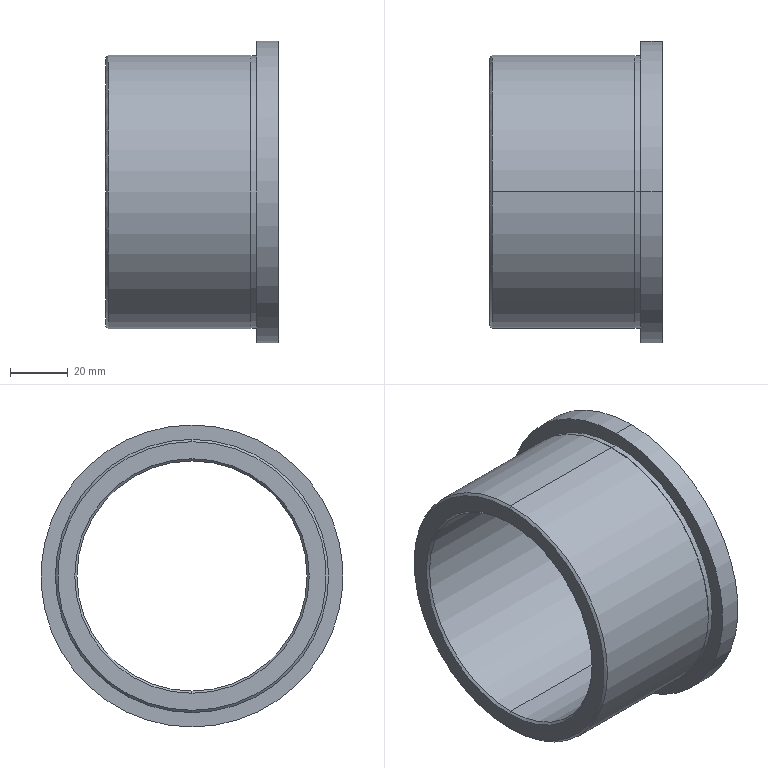Part | SolidWorks | features Revolution 1 | 1 solid | 18 faces | box 60 x 105 x 105 mm | volume 135111 mm3 | cylinder 8 | cone 6 | plane 4 | commonest cylinder face diameters 80 x2 94.6 x2 95 x2 105 x2
STEP:
#1=CARTESIAN_POINT('',(-30.,0.,46.7));
#2=VERTEX_POINT('',#1);
#3=CARTESIAN_POINT('',(-30.,0.,-46.7));
#4=VERTEX_POINT('',#3);
#5=CARTESIAN_POINT('',(-30.,0.,0.));
#6=DIRECTION('',(-1.,0.,0.));
#7=DIRECTION('',(0.,0.,1.));
#8=AXIS2_PLACEMENT_3D('',#5,#6,#7);
#9=CIRCLE('',#8,46.7);
#10=EDGE_CURVE('',#2,#4,#9,.T.);
#11=ORIENTED_EDGE('',*,*,#10,.F.);
#12=CARTESIAN_POINT('',(-29.2,0.,47.5));
#13=VERTEX_POINT('',#12);
#14=CARTESIAN_POINT('',(-29.2,0.,47.5));
#15=DIRECTION('',(0.7071,0.,0.7071));
#16=VECTOR('',#15,1000.);
#17=LINE('',#14,#16);
#18=EDGE_CURVE('',#2,#13,#17,.T.);
#19=ORIENTED_EDGE('',*,*,#18,.T.);
#20=CARTESIAN_POINT('',(-29.2,0.,-47.5));
#21=VERTEX_POINT('',#20);
#22=CARTESIAN_POINT('',(-29.2,0.,0.));
#23=DIRECTION('',(-1.,0.,0.));
#24=DIRECTION('',(0.,0.,1.));
#25=AXIS2_PLACEMENT_3D('',#22,#23,#24);
#26=CIRCLE('',#25,47.5);
#27=EDGE_CURVE('',#13,#21,#26,.T.);
#28=ORIENTED_EDGE('',*,*,#27,.T.);
#29=CARTESIAN_POINT('',(-29.2,0.,-47.5));
#30=DIRECTION('',(0.7071,0.,-0.7071));
#31=VECTOR('',#30,1000.);
#32=LINE('',#29,#31);
#33=EDGE_CURVE('',#4,#21,#32,.T.);
#34=ORIENTED_EDGE('',*,*,#33,.F.);
#35=EDGE_LOOP('',(#11,#19,#28,#34));
#36=FACE_OUTER_BOUND('',#35,.T.);
#37=CARTESIAN_POINT('',(-29.2,0.,0.));
#38=DIRECTION('',(1.,0.,0.));
#39=DIRECTION('',(0.,0.,-1.));
#40=AXIS2_PLACEMENT_3D('',#37,#38,#39);
#41=CONICAL_SURFACE('',#40,47.5,0.7854);
#42=ADVANCED_FACE('',(#36),#41,.T.);
#43=CARTESIAN_POINT('',(20.5,0.,47.5));
#44=VERTEX_POINT('',#43);
#45=CARTESIAN_POINT('',(20.5,0.,-47.5));
#46=VERTEX_POINT('',#45);
#47=CARTESIAN_POINT('',(20.5,0.,0.));
#48=DIRECTION('',(-1.,0.,0.));
#49=DIRECTION('',(0.,0.,1.));
#50=AXIS2_PLACEMENT_3D('',#47,#48,#49);
#51=CIRCLE('',#50,47.5);
#52=EDGE_CURVE('',#44,#46,#51,.T.);
#53=ORIENTED_EDGE('',*,*,#52,.T.);
#54=CARTESIAN_POINT('',(-30.,0.,-47.5));
#55=DIRECTION('',(-1.,0.,0.));
#56=VECTOR('',#55,1000.);
#57=LINE('',#54,#56);
#58=EDGE_CURVE('',#46,#21,#57,.T.);
#59=ORIENTED_EDGE('',*,*,#58,.T.);
#60=ORIENTED_EDGE('',*,*,#27,.F.);
#61=CARTESIAN_POINT('',(-30.,0.,47.5));
#62=DIRECTION('',(-1.,0.,0.));
#63=VECTOR('',#62,1000.);
#64=LINE('',#61,#63);
#65=EDGE_CURVE('',#44,#13,#64,.T.);
#66=ORIENTED_EDGE('',*,*,#65,.F.);
#67=EDGE_LOOP('',(#53,#59,#60,#66));
#68=FACE_OUTER_BOUND('',#67,.T.);
#69=CARTESIAN_POINT('',(-30.,0.,0.));
#70=DIRECTION('',(-1.,0.,0.));
#71=DIRECTION('',(0.,0.,1.));
#72=AXIS2_PLACEMENT_3D('',#69,#70,#71);
#73=CYLINDRICAL_SURFACE('',#72,47.5);
#74=ADVANCED_FACE('',(#68),#73,.T.);
#75=CARTESIAN_POINT('',(22.5,0.,47.3));
#76=VERTEX_POINT('',#75);
#77=CARTESIAN_POINT('',(22.5,0.,-47.3));
#78=VERTEX_POINT('',#77);
#79=CARTESIAN_POINT('',(22.5,0.,0.));
#80=DIRECTION('',(-1.,0.,0.));
#81=DIRECTION('',(0.,0.,1.));
#82=AXIS2_PLACEMENT_3D('',#79,#80,#81);
#83=CIRCLE('',#82,47.3);
#84=EDGE_CURVE('',#76,#78,#83,.T.);
#85=ORIENTED_EDGE('',*,*,#84,.T.);
#86=CARTESIAN_POINT('',(20.5,0.,-47.3));
#87=VERTEX_POINT('',#86);
#88=CARTESIAN_POINT('',(-30.,0.,-47.3));
#89=DIRECTION('',(-1.,0.,0.));
#90=VECTOR('',#89,1000.);
#91=LINE('',#88,#90);
#92=EDGE_CURVE('',#78,#87,#91,.T.);
#93=ORIENTED_EDGE('',*,*,#92,.T.);
#94=CARTESIAN_POINT('',(20.5,0.,47.3));
#95=VERTEX_POINT('',#94);
#96=CARTESIAN_POINT('',(20.5,0.,0.));
#97=DIRECTION('',(-1.,0.,0.));
#98=DIRECTION('',(0.,0.,1.));
#99=AXIS2_PLACEMENT_3D('',#96,#97,#98);
#100=CIRCLE('',#99,47.3);
#101=EDGE_CURVE('',#95,#87,#100,.T.);
#102=ORIENTED_EDGE('',*,*,#101,.F.);
#103=CARTESIAN_POINT('',(-30.,0.,47.3));
#104=DIRECTION('',(-1.,0.,0.));
#105=VECTOR('',#104,1000.);
#106=LINE('',#103,#105);
#107=EDGE_CURVE('',#76,#95,#106,.T.);
#108=ORIENTED_EDGE('',*,*,#107,.F.);
#109=EDGE_LOOP('',(#85,#93,#102,#108));
#110=FACE_OUTER_BOUND('',#109,.T.);
#111=CARTESIAN_POINT('',(-30.,0.,0.));
#112=DIRECTION('',(-1.,0.,0.));
#113=DIRECTION('',(0.,0.,1.));
#114=AXIS2_PLACEMENT_3D('',#111,#112,#113);
#115=CYLINDRICAL_SURFACE('',#114,47.3);
#116=ADVANCED_FACE('',(#110),#115,.T.);
#117=CARTESIAN_POINT('',(30.,0.,52.5));
#118=VERTEX_POINT('',#117);
#119=CARTESIAN_POINT('',(30.,0.,-52.5));
#120=VERTEX_POINT('',#119);
#121=CARTESIAN_POINT('',(30.,0.,0.));
#122=DIRECTION('',(-1.,0.,0.));
#123=DIRECTION('',(0.,0.,1.));
#124=AXIS2_PLACEMENT_3D('',#121,#122,#123);
#125=CIRCLE('',#124,52.5);
#126=EDGE_CURVE('',#118,#120,#125,.T.);
#127=ORIENTED_EDGE('',*,*,#126,.T.);
#128=CARTESIAN_POINT('',(22.5,0.,-52.5));
#129=VERTEX_POINT('',#128);
#130=CARTESIAN_POINT('',(-30.,0.,-52.5));
#131=DIRECTION('',(-1.,0.,0.));
#132=VECTOR('',#131,1000.);
#133=LINE('',#130,#132);
#134=EDGE_CURVE('',#120,#129,#133,.T.);
#135=ORIENTED_EDGE('',*,*,#134,.T.);
#136=CARTESIAN_POINT('',(22.5,0.,52.5));
#137=VERTEX_POINT('',#136);
#138=CARTESIAN_POINT('',(22.5,0.,0.));
#139=DIRECTION('',(-1.,0.,0.));
#140=DIRECTION('',(0.,0.,1.));
#141=AXIS2_PLACEMENT_3D('',#138,#139,#140);
#142=CIRCLE('',#141,52.5);
#143=EDGE_CURVE('',#137,#129,#142,.T.);
#144=ORIENTED_EDGE('',*,*,#143,.F.);
#145=CARTESIAN_POINT('',(-30.,0.,52.5));
#146=DIRECTION('',(-1.,0.,0.));
#147=VECTOR('',#146,1000.);
#148=LINE('',#145,#147);
#149=EDGE_CURVE('',#118,#137,#148,.T.);
#150=ORIENTED_EDGE('',*,*,#149,.F.);
#151=EDGE_LOOP('',(#127,#135,#144,#150));
#152=FACE_OUTER_BOUND('',#151,.T.);
#153=CARTESIAN_POINT('',(-30.,0.,0.));
#154=DIRECTION('',(-1.,0.,0.));
#155=DIRECTION('',(0.,0.,1.));
#156=AXIS2_PLACEMENT_3D('',#153,#154,#155);
#157=CYLINDRICAL_SURFACE('',#156,52.5);
#158=ADVANCED_FACE('',(#152),#157,.T.);
#159=CARTESIAN_POINT('',(29.2,0.,-40.));
#160=VERTEX_POINT('',#159);
#161=CARTESIAN_POINT('',(29.2,0.,40.));
#162=VERTEX_POINT('',#161);
#163=CARTESIAN_POINT('',(29.2,0.,0.));
#164=DIRECTION('',(-1.,0.,0.));
#165=DIRECTION('',(0.,0.,1.));
#166=AXIS2_PLACEMENT_3D('',#163,#164,#165);
#167=CIRCLE('',#166,40.);
#168=EDGE_CURVE('',#160,#162,#167,.T.);
#169=ORIENTED_EDGE('',*,*,#168,.T.);
#170=CARTESIAN_POINT('',(30.,0.,40.773));
#171=VERTEX_POINT('',#170);
#172=CARTESIAN_POINT('',(29.2,0.,40.));
#173=DIRECTION('',(0.7193,0.,0.6947));
#174=VECTOR('',#173,1000.);
#175=LINE('',#172,#174);
#176=EDGE_CURVE('',#162,#171,#175,.T.);
#177=ORIENTED_EDGE('',*,*,#176,.T.);
#178=CARTESIAN_POINT('',(30.,0.,-40.773));
#179=VERTEX_POINT('',#178);
#180=CARTESIAN_POINT('',(30.,0.,0.));
#181=DIRECTION('',(-1.,0.,0.));
#182=DIRECTION('',(0.,0.,1.));
#183=AXIS2_PLACEMENT_3D('',#180,#181,#182);
#184=CIRCLE('',#183,40.773);
#185=EDGE_CURVE('',#179,#171,#184,.T.);
#186=ORIENTED_EDGE('',*,*,#185,.F.);
#187=CARTESIAN_POINT('',(29.2,0.,-40.));
#188=DIRECTION('',(0.7193,0.,-0.6947));
#189=VECTOR('',#188,1000.);
#190=LINE('',#187,#189);
#191=EDGE_CURVE('',#160,#179,#190,.T.);
#192=ORIENTED_EDGE('',*,*,#191,.F.);
#193=EDGE_LOOP('',(#169,#177,#186,#192));
#194=FACE_OUTER_BOUND('',#193,.T.);
#195=CARTESIAN_POINT('',(29.2,0.,0.));
#196=DIRECTION('',(1.,0.,0.));
#197=DIRECTION('',(0.,0.,-1.));
#198=AXIS2_PLACEMENT_3D('',#195,#196,#197);
#199=CONICAL_SURFACE('',#198,40.,0.7679);
#200=ADVANCED_FACE('',(#194),#199,.F.);
#201=ORIENTED_EDGE('',*,*,#168,.F.);
#202=CARTESIAN_POINT('',(-29.2,0.,-40.));
#203=VERTEX_POINT('',#202);
#204=CARTESIAN_POINT('',(-30.,0.,-40.));
#205=DIRECTION('',(-1.,0.,0.));
#206=VECTOR('',#205,1000.);
#207=LINE('',#204,#206);
#208=EDGE_CURVE('',#160,#203,#207,.T.);
#209=ORIENTED_EDGE('',*,*,#208,.T.);
#210=CARTESIAN_POINT('',(-29.2,0.,40.));
#211=VERTEX_POINT('',#210);
#212=CARTESIAN_POINT('',(-29.2,0.,0.));
#213=DIRECTION('',(-1.,0.,0.));
#214=DIRECTION('',(0.,0.,1.));
#215=AXIS2_PLACEMENT_3D('',#212,#213,#214);
#216=CIRCLE('',#215,40.);
#217=EDGE_CURVE('',#203,#211,#216,.T.);
#218=ORIENTED_EDGE('',*,*,#217,.T.);
#219=CARTESIAN_POINT('',(-30.,0.,40.));
#220=DIRECTION('',(-1.,0.,0.));
#221=VECTOR('',#220,1000.);
#222=LINE('',#219,#221);
#223=EDGE_CURVE('',#162,#211,#222,.T.);
#224=ORIENTED_EDGE('',*,*,#223,.F.);
#225=EDGE_LOOP('',(#201,#209,#218,#224));
#226=FACE_OUTER_BOUND('',#225,.T.);
#227=CARTESIAN_POINT('',(-30.,0.,0.));
#228=DIRECTION('',(-1.,0.,0.));
#229=DIRECTION('',(0.,0.,1.));
#230=AXIS2_PLACEMENT_3D('',#227,#228,#229);
#231=CYLINDRICAL_SURFACE('',#230,40.);
#232=ADVANCED_FACE('',(#226),#231,.F.);
#233=ORIENTED_EDGE('',*,*,#217,.F.);
#234=CARTESIAN_POINT('',(-30.,0.,-40.773));
#235=VERTEX_POINT('',#234);
#236=CARTESIAN_POINT('',(-30.,0.,-40.773));
#237=DIRECTION('',(-0.7193,0.,-0.6947));
#238=VECTOR('',#237,1000.);
#239=LINE('',#236,#238);
#240=EDGE_CURVE('',#203,#235,#239,.T.);
#241=ORIENTED_EDGE('',*,*,#240,.T.);
#242=CARTESIAN_POINT('',(-30.,0.,40.773));
#243=VERTEX_POINT('',#242);
#244=CARTESIAN_POINT('',(-30.,0.,0.));
#245=DIRECTION('',(-1.,0.,0.));
#246=DIRECTION('',(0.,0.,1.));
#247=AXIS2_PLACEMENT_3D('',#244,#245,#246);
#248=CIRCLE('',#247,40.773);
#249=EDGE_CURVE('',#235,#243,#248,.T.);
#250=ORIENTED_EDGE('',*,*,#249,.T.);
#251=CARTESIAN_POINT('',(-30.,0.,40.773));
#252=DIRECTION('',(-0.7193,0.,0.6947));
#253=VECTOR('',#252,1000.);
#254=LINE('',#251,#253);
#255=EDGE_CURVE('',#211,#243,#254,.T.);
#256=ORIENTED_EDGE('',*,*,#255,.F.);
#257=EDGE_LOOP('',(#233,#241,#250,#256));
#258=FACE_OUTER_BOUND('',#257,.T.);
#259=CARTESIAN_POINT('',(-30.,0.,0.));
#260=DIRECTION('',(-1.,0.,0.));
#261=DIRECTION('',(0.,0.,1.));
#262=AXIS2_PLACEMENT_3D('',#259,#260,#261);
#263=CONICAL_SURFACE('',#262,40.773,0.7679);
#264=ADVANCED_FACE('',(#258),#263,.F.);
#265=CARTESIAN_POINT('',(-30.,0.,0.));
#266=DIRECTION('',(-1.,0.,0.));
#267=DIRECTION('',(0.,0.,1.));
#268=AXIS2_PLACEMENT_3D('',#265,#266,#267);
#269=CIRCLE('',#268,40.773);
#270=EDGE_CURVE('',#243,#235,#269,.T.);
#271=ORIENTED_EDGE('',*,*,#270,.F.);
#272=ORIENTED_EDGE('',*,*,#249,.F.);
#273=EDGE_LOOP('',(#271,#272));
#274=FACE_BOUND('',#273,.T.);
#275=CARTESIAN_POINT('',(-30.,0.,0.));
#276=DIRECTION('',(-1.,0.,0.));
#277=DIRECTION('',(0.,0.,1.));
#278=AXIS2_PLACEMENT_3D('',#275,#276,#277);
#279=CIRCLE('',#278,46.7);
#280=EDGE_CURVE('',#4,#2,#279,.T.);
#281=ORIENTED_EDGE('',*,*,#280,.T.);
#282=ORIENTED_EDGE('',*,*,#10,.T.);
#283=EDGE_LOOP('',(#281,#282));
#284=FACE_OUTER_BOUND('',#283,.T.);
#285=CARTESIAN_POINT('',(-30.,46.7,0.));
#286=DIRECTION('',(1.,0.,0.));
#287=DIRECTION('',(0.,0.,-1.));
#288=AXIS2_PLACEMENT_3D('',#285,#286,#287);
#289=PLANE('',#288);
#290=ADVANCED_FACE('',(#274,#284),#289,.F.);
#291=ORIENTED_EDGE('',*,*,#240,.F.);
#292=CARTESIAN_POINT('',(-29.2,0.,0.));
#293=DIRECTION('',(-1.,0.,0.));
#294=DIRECTION('',(0.,0.,1.));
#295=AXIS2_PLACEMENT_3D('',#292,#293,#294);
#296=CIRCLE('',#295,40.);
#297=EDGE_CURVE('',#211,#203,#296,.T.);
#298=ORIENTED_EDGE('',*,*,#297,.F.);
#299=ORIENTED_EDGE('',*,*,#255,.T.);
#300=ORIENTED_EDGE('',*,*,#270,.T.);
#301=EDGE_LOOP('',(#291,#298,#299,#300));
#302=FACE_OUTER_BOUND('',#301,.T.);
#303=CARTESIAN_POINT('',(-30.,0.,0.));
#304=DIRECTION('',(-1.,0.,0.));
#305=DIRECTION('',(0.,0.,1.));
#306=AXIS2_PLACEMENT_3D('',#303,#304,#305);
#307=CONICAL_SURFACE('',#306,40.773,0.7679);
#308=ADVANCED_FACE('',(#302),#307,.F.);
#309=ORIENTED_EDGE('',*,*,#208,.F.);
#310=CARTESIAN_POINT('',(29.2,0.,0.));
#311=DIRECTION('',(-1.,0.,0.));
#312=DIRECTION('',(0.,0.,1.));
#313=AXIS2_PLACEMENT_3D('',#310,#311,#312);
#314=CIRCLE('',#313,40.);
#315=EDGE_CURVE('',#162,#160,#314,.T.);
#316=ORIENTED_EDGE('',*,*,#315,.F.);
#317=ORIENTED_EDGE('',*,*,#223,.T.);
#318=ORIENTED_EDGE('',*,*,#297,.T.);
#319=EDGE_LOOP('',(#309,#316,#317,#318));
#320=FACE_OUTER_BOUND('',#319,.T.);
#321=CARTESIAN_POINT('',(-30.,0.,0.));
#322=DIRECTION('',(-1.,0.,0.));
#323=DIRECTION('',(0.,0.,1.));
#324=AXIS2_PLACEMENT_3D('',#321,#322,#323);
#325=CYLINDRICAL_SURFACE('',#324,40.);
#326=ADVANCED_FACE('',(#320),#325,.F.);
#327=ORIENTED_EDGE('',*,*,#176,.F.);
#328=ORIENTED_EDGE('',*,*,#315,.T.);
#329=ORIENTED_EDGE('',*,*,#191,.T.);
#330=CARTESIAN_POINT('',(30.,0.,0.));
#331=DIRECTION('',(-1.,0.,0.));
#332=DIRECTION('',(0.,0.,1.));
#333=AXIS2_PLACEMENT_3D('',#330,#331,#332);
#334=CIRCLE('',#333,40.773);
#335=EDGE_CURVE('',#171,#179,#334,.T.);
#336=ORIENTED_EDGE('',*,*,#335,.F.);
#337=EDGE_LOOP('',(#327,#328,#329,#336));
#338=FACE_OUTER_BOUND('',#337,.T.);
#339=CARTESIAN_POINT('',(29.2,0.,0.));
#340=DIRECTION('',(1.,0.,0.));
#341=DIRECTION('',(0.,0.,-1.));
#342=AXIS2_PLACEMENT_3D('',#339,#340,#341);
#343=CONICAL_SURFACE('',#342,40.,0.7679);
#344=ADVANCED_FACE('',(#338),#343,.F.);
#345=ORIENTED_EDGE('',*,*,#126,.F.);
#346=CARTESIAN_POINT('',(30.,0.,0.));
#347=DIRECTION('',(-1.,0.,0.));
#348=DIRECTION('',(0.,0.,1.));
#349=AXIS2_PLACEMENT_3D('',#346,#347,#348);
#350=CIRCLE('',#349,52.5);
#351=EDGE_CURVE('',#120,#118,#350,.T.);
#352=ORIENTED_EDGE('',*,*,#351,.F.);
#353=EDGE_LOOP('',(#345,#352));
#354=FACE_OUTER_BOUND('',#353,.T.);
#355=ORIENTED_EDGE('',*,*,#185,.T.);
#356=ORIENTED_EDGE('',*,*,#335,.T.);
#357=EDGE_LOOP('',(#355,#356));
#358=FACE_BOUND('',#357,.T.);
#359=CARTESIAN_POINT('',(30.,40.773,0.));
#360=DIRECTION('',(-1.,0.,0.));
#361=DIRECTION('',(0.,0.,1.));
#362=AXIS2_PLACEMENT_3D('',#359,#360,#361);
#363=PLANE('',#362);
#364=ADVANCED_FACE('',(#354,#358),#363,.F.);
#365=ORIENTED_EDGE('',*,*,#134,.F.);
#366=ORIENTED_EDGE('',*,*,#351,.T.);
#367=ORIENTED_EDGE('',*,*,#149,.T.);
#368=CARTESIAN_POINT('',(22.5,0.,0.));
#369=DIRECTION('',(-1.,0.,0.));
#370=DIRECTION('',(0.,0.,1.));
#371=AXIS2_PLACEMENT_3D('',#368,#369,#370);
#372=CIRCLE('',#371,52.5);
#373=EDGE_CURVE('',#129,#137,#372,.T.);
#374=ORIENTED_EDGE('',*,*,#373,.F.);
#375=EDGE_LOOP('',(#365,#366,#367,#374));
#376=FACE_OUTER_BOUND('',#375,.T.);
#377=CARTESIAN_POINT('',(-30.,0.,0.));
#378=DIRECTION('',(-1.,0.,0.));
#379=DIRECTION('',(0.,0.,1.));
#380=AXIS2_PLACEMENT_3D('',#377,#378,#379);
#381=CYLINDRICAL_SURFACE('',#380,52.5);
#382=ADVANCED_FACE('',(#376),#381,.T.);
#383=ORIENTED_EDGE('',*,*,#84,.F.);
#384=CARTESIAN_POINT('',(22.5,0.,0.));
#385=DIRECTION('',(-1.,0.,0.));
#386=DIRECTION('',(0.,0.,1.));
#387=AXIS2_PLACEMENT_3D('',#384,#385,#386);
#388=CIRCLE('',#387,47.3);
#389=EDGE_CURVE('',#78,#76,#388,.T.);
#390=ORIENTED_EDGE('',*,*,#389,.F.);
#391=EDGE_LOOP('',(#383,#390));
#392=FACE_BOUND('',#391,.T.);
#393=ORIENTED_EDGE('',*,*,#143,.T.);
#394=ORIENTED_EDGE('',*,*,#373,.T.);
#395=EDGE_LOOP('',(#393,#394));
#396=FACE_OUTER_BOUND('',#395,.T.);
#397=CARTESIAN_POINT('',(22.5,52.5,0.));
#398=DIRECTION('',(1.,0.,0.));
#399=DIRECTION('',(0.,0.,-1.));
#400=AXIS2_PLACEMENT_3D('',#397,#398,#399);
#401=PLANE('',#400);
#402=ADVANCED_FACE('',(#392,#396),#401,.F.);
#403=ORIENTED_EDGE('',*,*,#92,.F.);
#404=ORIENTED_EDGE('',*,*,#389,.T.);
#405=ORIENTED_EDGE('',*,*,#107,.T.);
#406=CARTESIAN_POINT('',(20.5,0.,0.));
#407=DIRECTION('',(-1.,0.,0.));
#408=DIRECTION('',(0.,0.,1.));
#409=AXIS2_PLACEMENT_3D('',#406,#407,#408);
#410=CIRCLE('',#409,47.3);
#411=EDGE_CURVE('',#87,#95,#410,.T.);
#412=ORIENTED_EDGE('',*,*,#411,.F.);
#413=EDGE_LOOP('',(#403,#404,#405,#412));
#414=FACE_OUTER_BOUND('',#413,.T.);
#415=CARTESIAN_POINT('',(-30.,0.,0.));
#416=DIRECTION('',(-1.,0.,0.));
#417=DIRECTION('',(0.,0.,1.));
#418=AXIS2_PLACEMENT_3D('',#415,#416,#417);
#419=CYLINDRICAL_SURFACE('',#418,47.3);
#420=ADVANCED_FACE('',(#414),#419,.T.);
#421=ORIENTED_EDGE('',*,*,#52,.F.);
#422=CARTESIAN_POINT('',(20.5,0.,0.));
#423=DIRECTION('',(-1.,0.,0.));
#424=DIRECTION('',(0.,0.,1.));
#425=AXIS2_PLACEMENT_3D('',#422,#423,#424);
#426=CIRCLE('',#425,47.5);
#427=EDGE_CURVE('',#46,#44,#426,.T.);
#428=ORIENTED_EDGE('',*,*,#427,.F.);
#429=EDGE_LOOP('',(#421,#428));
#430=FACE_OUTER_BOUND('',#429,.T.);
#431=ORIENTED_EDGE('',*,*,#101,.T.);
#432=ORIENTED_EDGE('',*,*,#411,.T.);
#433=EDGE_LOOP('',(#431,#432));
#434=FACE_BOUND('',#433,.T.);
#435=CARTESIAN_POINT('',(20.5,47.3,0.));
#436=DIRECTION('',(-1.,0.,0.));
#437=DIRECTION('',(0.,0.,1.));
#438=AXIS2_PLACEMENT_3D('',#435,#436,#437);
#439=PLANE('',#438);
#440=ADVANCED_FACE('',(#430,#434),#439,.F.);
#441=ORIENTED_EDGE('',*,*,#58,.F.);
#442=ORIENTED_EDGE('',*,*,#427,.T.);
#443=ORIENTED_EDGE('',*,*,#65,.T.);
#444=CARTESIAN_POINT('',(-29.2,0.,0.));
#445=DIRECTION('',(-1.,0.,0.));
#446=DIRECTION('',(0.,0.,1.));
#447=AXIS2_PLACEMENT_3D('',#444,#445,#446);
#448=CIRCLE('',#447,47.5);
#449=EDGE_CURVE('',#21,#13,#448,.T.);
#450=ORIENTED_EDGE('',*,*,#449,.F.);
#451=EDGE_LOOP('',(#441,#442,#443,#450));
#452=FACE_OUTER_BOUND('',#451,.T.);
#453=CARTESIAN_POINT('',(-30.,0.,0.));
#454=DIRECTION('',(-1.,0.,0.));
#455=DIRECTION('',(0.,0.,1.));
#456=AXIS2_PLACEMENT_3D('',#453,#454,#455);
#457=CYLINDRICAL_SURFACE('',#456,47.5);
#458=ADVANCED_FACE('',(#452),#457,.T.);
#459=ORIENTED_EDGE('',*,*,#18,.F.);
#460=ORIENTED_EDGE('',*,*,#280,.F.);
#461=ORIENTED_EDGE('',*,*,#33,.T.);
#462=ORIENTED_EDGE('',*,*,#449,.T.);
#463=EDGE_LOOP('',(#459,#460,#461,#462));
#464=FACE_OUTER_BOUND('',#463,.T.);
#465=CARTESIAN_POINT('',(-29.2,0.,0.));
#466=DIRECTION('',(1.,0.,0.));
#467=DIRECTION('',(0.,0.,-1.));
#468=AXIS2_PLACEMENT_3D('',#465,#466,#467);
#469=CONICAL_SURFACE('',#468,47.5,0.7854);
#470=ADVANCED_FACE('',(#464),#469,.T.);
#471=CLOSED_SHELL('',(#42,#74,#116,#158,#200,#232,#264,#290,#308,#326,#344,#364,#382,#402,#420,#440,#458,#470));
#472=MANIFOLD_SOLID_BREP('',#471);
#473=CARTESIAN_POINT('',(0.,0.,0.));
#474=DIRECTION('',(0.,0.,1.));
#475=DIRECTION('',(1.,0.,0.));
#476=AXIS2_PLACEMENT_3D('',#473,#474,#475);
#477=(LENGTH_UNIT()NAMED_UNIT(*)SI_UNIT(.MILLI.,.METRE.));
#478=UNCERTAINTY_MEASURE_WITH_UNIT(LENGTH_MEASURE(0.00001),#477,'','');
#479=(NAMED_UNIT(*)PLANE_ANGLE_UNIT()SI_UNIT($,.RADIAN.));
#480=(NAMED_UNIT(*)SI_UNIT($,.STERADIAN.)SOLID_ANGLE_UNIT());
#481=(GEOMETRIC_REPRESENTATION_CONTEXT(3)GLOBAL_UNCERTAINTY_ASSIGNED_CONTEXT((#478))GLOBAL_UNIT_ASSIGNED_CONTEXT((#477,#479,#480))REPRESENTATION_CONTEXT('',''));
#482=ADVANCED_BREP_SHAPE_REPRESENTATION('',(#472,#476),#481);